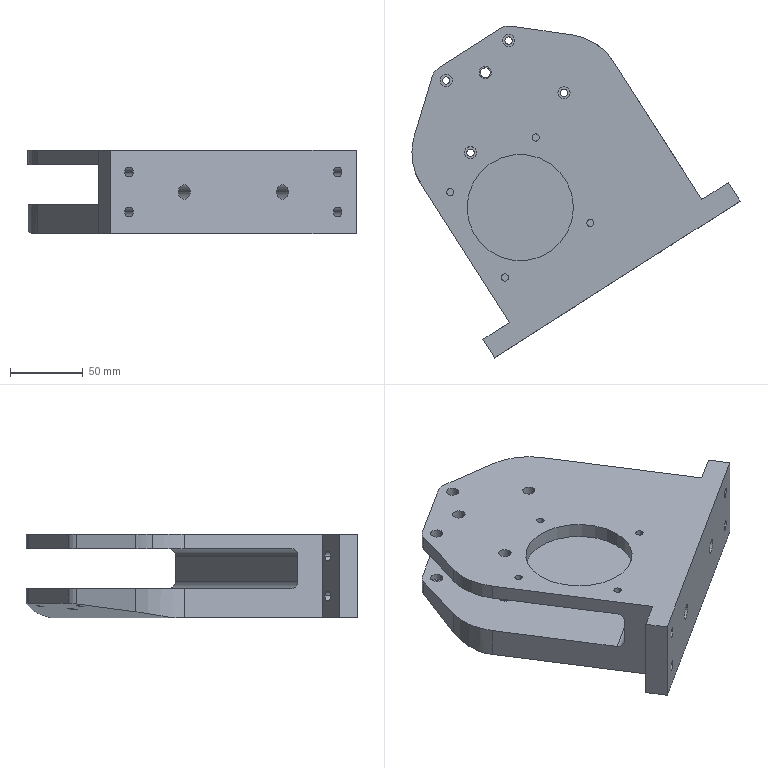Part | SolidWorks | features Cut 5, HoleWzd 5, ICE 3, Extrusion 1, Fillet 1 | 1 solid | 88 faces | box 225.335 x 227.919 x 57.4 mm | volume 931418 mm3 | cylinder 61 | plane 23 | cone 4 | commonest cylinder face diameters 5 x16 8.382 x16 6.8 x10 10 x6 80.433 x5 20 x4